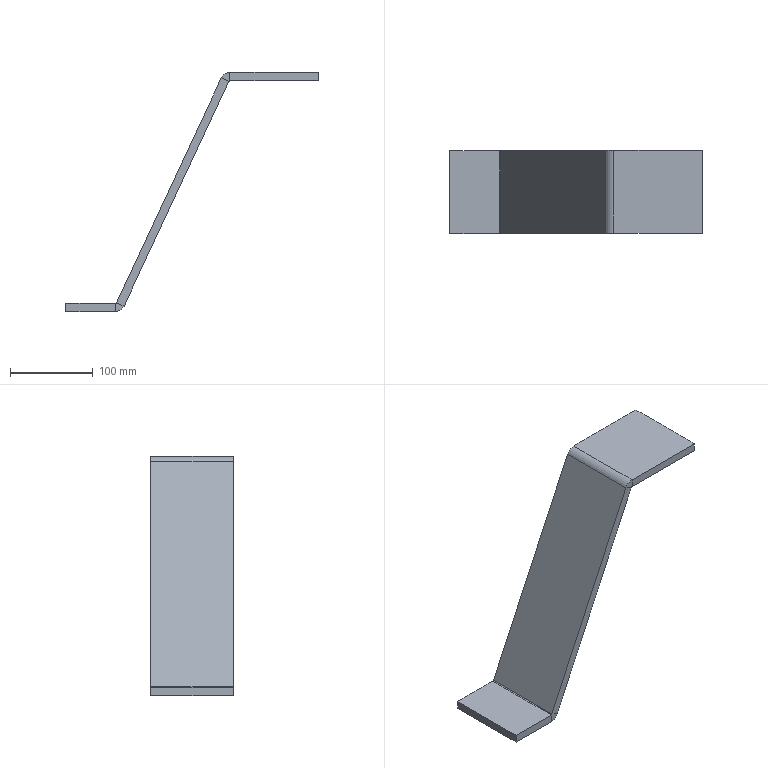Part | STEP file | B1 | 1 solid | 22 faces | box 305.057 x 100 x 289.003 mm | volume 480985 mm3 | plane 18 | cylinder 4 | commonest cylinder face diameters 3 x2 23 x2
STEP:
#1=CARTESIAN_POINT('',(0.,0.,0.));
#2=DIRECTION('',(0.,0.,1.));
#3=DIRECTION('',(1.,0.,0.));
#4=AXIS2_PLACEMENT_3D('',#1,#2,#3);
#5=CARTESIAN_POINT('',(0.,100.,0.));
#6=VERTEX_POINT('',#5);
#7=CARTESIAN_POINT('',(0.,0.,0.));
#8=VERTEX_POINT('',#7);
#9=CARTESIAN_POINT('',(0.,100.,0.));
#10=DIRECTION('',(0.,-1.,0.));
#11=VECTOR('',#10,1.);
#12=LINE('',#9,#11);
#13=CARTESIAN_POINT('',(0.,100.,-10.));
#14=DIRECTION('',(-1.,0.,0.));
#15=DIRECTION('',(0.,-1.,0.));
#16=AXIS2_PLACEMENT_3D('',#13,#14,#15);
#17=PLANE('',#16);
#18=CARTESIAN_POINT('',(0.,10.));
#19=DIRECTION('',(1.,0.));
#20=VECTOR('',#19,1.);
#21=LINE('',#18,#20);
#22=(GEOMETRIC_REPRESENTATION_CONTEXT(2)PARAMETRIC_REPRESENTATION_CONTEXT()REPRESENTATION_CONTEXT('',''));
#23=DEFINITIONAL_REPRESENTATION('',(#21),#22);
#24=PCURVE('',#17,#23);
#25=CARTESIAN_POINT('',(0.,0.,0.));
#26=DIRECTION('',(0.,0.,1.));
#27=DIRECTION('',(1.,0.,0.));
#28=AXIS2_PLACEMENT_3D('',#25,#26,#27);
#29=PLANE('',#28);
#30=CARTESIAN_POINT('',(0.,100.));
#31=DIRECTION('',(0.,-1.));
#32=VECTOR('',#31,1.);
#33=LINE('',#30,#32);
#34=(GEOMETRIC_REPRESENTATION_CONTEXT(2)PARAMETRIC_REPRESENTATION_CONTEXT()REPRESENTATION_CONTEXT('',''));
#35=DEFINITIONAL_REPRESENTATION('',(#33),#34);
#36=PCURVE('',#29,#35);
#37=SURFACE_CURVE('',#12,(#24,#36),.PCURVE_S1.);
#38=EDGE_CURVE('',#6,#8,#37,.T.);
#39=ORIENTED_EDGE('',*,*,#38,.F.);
#40=CARTESIAN_POINT('',(0.,100.,-10.));
#41=VERTEX_POINT('',#40);
#42=CARTESIAN_POINT('',(0.,100.,-10.));
#43=DIRECTION('',(0.,0.,1.));
#44=VECTOR('',#43,1.);
#45=LINE('',#42,#44);
#46=CARTESIAN_POINT('',(0.,0.));
#47=DIRECTION('',(0.,1.));
#48=VECTOR('',#47,1.);
#49=LINE('',#46,#48);
#50=(GEOMETRIC_REPRESENTATION_CONTEXT(2)PARAMETRIC_REPRESENTATION_CONTEXT()REPRESENTATION_CONTEXT('',''));
#51=DEFINITIONAL_REPRESENTATION('',(#49),#50);
#52=PCURVE('',#17,#51);
#53=CARTESIAN_POINT('',(0.,100.,-10.));
#54=DIRECTION('',(0.,1.,0.));
#55=DIRECTION('',(-1.,0.,0.));
#56=AXIS2_PLACEMENT_3D('',#53,#54,#55);
#57=PLANE('',#56);
#58=CARTESIAN_POINT('',(0.,0.));
#59=DIRECTION('',(0.,1.));
#60=VECTOR('',#59,1.);
#61=LINE('',#58,#60);
#62=(GEOMETRIC_REPRESENTATION_CONTEXT(2)PARAMETRIC_REPRESENTATION_CONTEXT()REPRESENTATION_CONTEXT('',''));
#63=DEFINITIONAL_REPRESENTATION('',(#61),#62);
#64=PCURVE('',#57,#63);
#65=SURFACE_CURVE('',#45,(#52,#64),.PCURVE_S1.);
#66=EDGE_CURVE('',#41,#6,#65,.T.);
#67=ORIENTED_EDGE('',*,*,#66,.F.);
#68=CARTESIAN_POINT('',(0.,0.,-10.));
#69=VERTEX_POINT('',#68);
#70=CARTESIAN_POINT('',(0.,100.,-10.));
#71=DIRECTION('',(0.,-1.,0.));
#72=VECTOR('',#71,1.);
#73=LINE('',#70,#72);
#74=CARTESIAN_POINT('',(0.,0.));
#75=DIRECTION('',(1.,0.));
#76=VECTOR('',#75,1.);
#77=LINE('',#74,#76);
#78=(GEOMETRIC_REPRESENTATION_CONTEXT(2)PARAMETRIC_REPRESENTATION_CONTEXT()REPRESENTATION_CONTEXT('',''));
#79=DEFINITIONAL_REPRESENTATION('',(#77),#78);
#80=PCURVE('',#17,#79);
#81=CARTESIAN_POINT('',(0.,0.,-10.));
#82=DIRECTION('',(0.,0.,1.));
#83=DIRECTION('',(1.,0.,0.));
#84=AXIS2_PLACEMENT_3D('',#81,#82,#83);
#85=PLANE('',#84);
#86=CARTESIAN_POINT('',(0.,100.));
#87=DIRECTION('',(0.,-1.));
#88=VECTOR('',#87,1.);
#89=LINE('',#86,#88);
#90=(GEOMETRIC_REPRESENTATION_CONTEXT(2)PARAMETRIC_REPRESENTATION_CONTEXT()REPRESENTATION_CONTEXT('',''));
#91=DEFINITIONAL_REPRESENTATION('',(#89),#90);
#92=PCURVE('',#85,#91);
#93=SURFACE_CURVE('',#73,(#80,#92),.PCURVE_S1.);
#94=EDGE_CURVE('',#41,#69,#93,.T.);
#95=ORIENTED_EDGE('',*,*,#94,.T.);
#96=CARTESIAN_POINT('',(0.,0.,-10.));
#97=DIRECTION('',(0.,0.,1.));
#98=VECTOR('',#97,1.);
#99=LINE('',#96,#98);
#100=CARTESIAN_POINT('',(100.,0.));
#101=DIRECTION('',(0.,1.));
#102=VECTOR('',#101,1.);
#103=LINE('',#100,#102);
#104=(GEOMETRIC_REPRESENTATION_CONTEXT(2)PARAMETRIC_REPRESENTATION_CONTEXT()REPRESENTATION_CONTEXT('',''));
#105=DEFINITIONAL_REPRESENTATION('',(#103),#104);
#106=PCURVE('',#17,#105);
#107=CARTESIAN_POINT('',(0.,0.,-10.));
#108=DIRECTION('',(0.,-1.,0.));
#109=DIRECTION('',(1.,0.,0.));
#110=AXIS2_PLACEMENT_3D('',#107,#108,#109);
#111=PLANE('',#110);
#112=CARTESIAN_POINT('',(0.,0.));
#113=DIRECTION('',(0.,1.));
#114=VECTOR('',#113,1.);
#115=LINE('',#112,#114);
#116=(GEOMETRIC_REPRESENTATION_CONTEXT(2)PARAMETRIC_REPRESENTATION_CONTEXT()REPRESENTATION_CONTEXT('',''));
#117=DEFINITIONAL_REPRESENTATION('',(#115),#116);
#118=PCURVE('',#111,#117);
#119=SURFACE_CURVE('',#99,(#106,#118),.PCURVE_S1.);
#120=EDGE_CURVE('',#69,#8,#119,.T.);
#121=ORIENTED_EDGE('',*,*,#120,.T.);
#122=EDGE_LOOP('',(#39,#67,#95,#121));
#123=FACE_BOUND('',#122,.T.);
#124=ADVANCED_FACE('',(#123),#17,.T.);
#125=CARTESIAN_POINT('',(60.,100.,0.));
#126=VERTEX_POINT('',#125);
#127=CARTESIAN_POINT('',(0.,100.,0.));
#128=DIRECTION('',(-1.,0.,0.));
#129=VECTOR('',#128,1.);
#130=LINE('',#127,#129);
#131=CARTESIAN_POINT('',(0.,10.));
#132=DIRECTION('',(1.,0.));
#133=VECTOR('',#132,1.);
#134=LINE('',#131,#133);
#135=(GEOMETRIC_REPRESENTATION_CONTEXT(2)PARAMETRIC_REPRESENTATION_CONTEXT()REPRESENTATION_CONTEXT('',''));
#136=DEFINITIONAL_REPRESENTATION('',(#134),#135);
#137=PCURVE('',#57,#136);
#138=CARTESIAN_POINT('',(0.,100.));
#139=DIRECTION('',(-1.,0.));
#140=VECTOR('',#139,1.);
#141=LINE('',#138,#140);
#142=(GEOMETRIC_REPRESENTATION_CONTEXT(2)PARAMETRIC_REPRESENTATION_CONTEXT()REPRESENTATION_CONTEXT('',''));
#143=DEFINITIONAL_REPRESENTATION('',(#141),#142);
#144=PCURVE('',#29,#143);
#145=SURFACE_CURVE('',#130,(#137,#144),.PCURVE_S1.);
#146=EDGE_CURVE('',#126,#6,#145,.T.);
#147=ORIENTED_EDGE('',*,*,#146,.F.);
#148=CARTESIAN_POINT('',(60.,100.,-10.));
#149=VERTEX_POINT('',#148);
#150=CARTESIAN_POINT('',(60.,100.,-10.));
#151=DIRECTION('',(0.,0.,1.));
#152=VECTOR('',#151,1.);
#153=LINE('',#150,#152);
#154=CARTESIAN_POINT('',(-60.,0.));
#155=DIRECTION('',(0.,1.));
#156=VECTOR('',#155,1.);
#157=LINE('',#154,#156);
#158=(GEOMETRIC_REPRESENTATION_CONTEXT(2)PARAMETRIC_REPRESENTATION_CONTEXT()REPRESENTATION_CONTEXT('',''));
#159=DEFINITIONAL_REPRESENTATION('',(#157),#158);
#160=PCURVE('',#57,#159);
#161=CARTESIAN_POINT('',(60.,100.,1.5));
#162=DIRECTION('',(0.,-1.,0.));
#163=DIRECTION('',(1.,0.,0.));
#164=AXIS2_PLACEMENT_3D('',#161,#162,#163);
#165=PLANE('',#164);
#166=CARTESIAN_POINT('',(0.,-11.5));
#167=DIRECTION('',(0.,1.));
#168=VECTOR('',#167,1.);
#169=LINE('',#166,#168);
#170=(GEOMETRIC_REPRESENTATION_CONTEXT(2)PARAMETRIC_REPRESENTATION_CONTEXT()REPRESENTATION_CONTEXT('',''));
#171=DEFINITIONAL_REPRESENTATION('',(#169),#170);
#172=PCURVE('',#165,#171);
#173=SURFACE_CURVE('',#153,(#160,#172),.PCURVE_S1.);
#174=EDGE_CURVE('',#149,#126,#173,.T.);
#175=ORIENTED_EDGE('',*,*,#174,.F.);
#176=CARTESIAN_POINT('',(0.,100.,-10.));
#177=DIRECTION('',(-1.,0.,0.));
#178=VECTOR('',#177,1.);
#179=LINE('',#176,#178);
#180=CARTESIAN_POINT('',(0.,0.));
#181=DIRECTION('',(1.,0.));
#182=VECTOR('',#181,1.);
#183=LINE('',#180,#182);
#184=(GEOMETRIC_REPRESENTATION_CONTEXT(2)PARAMETRIC_REPRESENTATION_CONTEXT()REPRESENTATION_CONTEXT('',''));
#185=DEFINITIONAL_REPRESENTATION('',(#183),#184);
#186=PCURVE('',#57,#185);
#187=CARTESIAN_POINT('',(0.,100.));
#188=DIRECTION('',(-1.,0.));
#189=VECTOR('',#188,1.);
#190=LINE('',#187,#189);
#191=(GEOMETRIC_REPRESENTATION_CONTEXT(2)PARAMETRIC_REPRESENTATION_CONTEXT()REPRESENTATION_CONTEXT('',''));
#192=DEFINITIONAL_REPRESENTATION('',(#190),#191);
#193=PCURVE('',#85,#192);
#194=SURFACE_CURVE('',#179,(#186,#193),.PCURVE_S1.);
#195=EDGE_CURVE('',#149,#41,#194,.T.);
#196=ORIENTED_EDGE('',*,*,#195,.T.);
#197=ORIENTED_EDGE('',*,*,#66,.T.);
#198=EDGE_LOOP('',(#147,#175,#196,#197));
#199=FACE_BOUND('',#198,.T.);
#200=ADVANCED_FACE('',(#199),#57,.T.);
#201=CARTESIAN_POINT('',(60.,0.,0.));
#202=VERTEX_POINT('',#201);
#203=CARTESIAN_POINT('',(0.,0.,0.));
#204=DIRECTION('',(1.,0.,0.));
#205=VECTOR('',#204,1.);
#206=LINE('',#203,#205);
#207=CARTESIAN_POINT('',(0.,10.));
#208=DIRECTION('',(1.,0.));
#209=VECTOR('',#208,1.);
#210=LINE('',#207,#209);
#211=(GEOMETRIC_REPRESENTATION_CONTEXT(2)PARAMETRIC_REPRESENTATION_CONTEXT()REPRESENTATION_CONTEXT('',''));
#212=DEFINITIONAL_REPRESENTATION('',(#210),#211);
#213=PCURVE('',#111,#212);
#214=CARTESIAN_POINT('',(0.,0.));
#215=DIRECTION('',(1.,0.));
#216=VECTOR('',#215,1.);
#217=LINE('',#214,#216);
#218=(GEOMETRIC_REPRESENTATION_CONTEXT(2)PARAMETRIC_REPRESENTATION_CONTEXT()REPRESENTATION_CONTEXT('',''));
#219=DEFINITIONAL_REPRESENTATION('',(#217),#218);
#220=PCURVE('',#29,#219);
#221=SURFACE_CURVE('',#206,(#213,#220),.PCURVE_S1.);
#222=EDGE_CURVE('',#8,#202,#221,.T.);
#223=ORIENTED_EDGE('',*,*,#222,.F.);
#224=ORIENTED_EDGE('',*,*,#120,.F.);
#225=CARTESIAN_POINT('',(60.,0.,-10.));
#226=VERTEX_POINT('',#225);
#227=CARTESIAN_POINT('',(0.,0.,-10.));
#228=DIRECTION('',(1.,0.,0.));
#229=VECTOR('',#228,1.);
#230=LINE('',#227,#229);
#231=CARTESIAN_POINT('',(0.,0.));
#232=DIRECTION('',(1.,0.));
#233=VECTOR('',#232,1.);
#234=LINE('',#231,#233);
#235=(GEOMETRIC_REPRESENTATION_CONTEXT(2)PARAMETRIC_REPRESENTATION_CONTEXT()REPRESENTATION_CONTEXT('',''));
#236=DEFINITIONAL_REPRESENTATION('',(#234),#235);
#237=PCURVE('',#111,#236);
#238=CARTESIAN_POINT('',(0.,0.));
#239=DIRECTION('',(1.,0.));
#240=VECTOR('',#239,1.);
#241=LINE('',#238,#240);
#242=(GEOMETRIC_REPRESENTATION_CONTEXT(2)PARAMETRIC_REPRESENTATION_CONTEXT()REPRESENTATION_CONTEXT('',''));
#243=DEFINITIONAL_REPRESENTATION('',(#241),#242);
#244=PCURVE('',#85,#243);
#245=SURFACE_CURVE('',#230,(#237,#244),.PCURVE_S1.);
#246=EDGE_CURVE('',#69,#226,#245,.T.);
#247=ORIENTED_EDGE('',*,*,#246,.T.);
#248=CARTESIAN_POINT('',(60.,0.,-10.));
#249=DIRECTION('',(0.,0.,1.));
#250=VECTOR('',#249,1.);
#251=LINE('',#248,#250);
#252=CARTESIAN_POINT('',(60.,0.));
#253=DIRECTION('',(0.,1.));
#254=VECTOR('',#253,1.);
#255=LINE('',#252,#254);
#256=(GEOMETRIC_REPRESENTATION_CONTEXT(2)PARAMETRIC_REPRESENTATION_CONTEXT()REPRESENTATION_CONTEXT('',''));
#257=DEFINITIONAL_REPRESENTATION('',(#255),#256);
#258=PCURVE('',#111,#257);
#259=CARTESIAN_POINT('',(60.,0.,1.5));
#260=DIRECTION('',(0.,-1.,0.));
#261=DIRECTION('',(1.,0.,0.));
#262=AXIS2_PLACEMENT_3D('',#259,#260,#261);
#263=PLANE('',#262);
#264=CARTESIAN_POINT('',(0.,-11.5));
#265=DIRECTION('',(0.,1.));
#266=VECTOR('',#265,1.);
#267=LINE('',#264,#266);
#268=(GEOMETRIC_REPRESENTATION_CONTEXT(2)PARAMETRIC_REPRESENTATION_CONTEXT()REPRESENTATION_CONTEXT('',''));
#269=DEFINITIONAL_REPRESENTATION('',(#267),#268);
#270=PCURVE('',#263,#269);
#271=SURFACE_CURVE('',#251,(#258,#270),.PCURVE_S1.);
#272=EDGE_CURVE('',#226,#202,#271,.T.);
#273=ORIENTED_EDGE('',*,*,#272,.T.);
#274=EDGE_LOOP('',(#223,#224,#247,#273));
#275=FACE_BOUND('',#274,.T.);
#276=ADVANCED_FACE('',(#275),#111,.T.);
#277=ORIENTED_EDGE('',*,*,#94,.F.);
#278=ORIENTED_EDGE('',*,*,#195,.F.);
#279=CARTESIAN_POINT('',(60.,100.,-10.));
#280=DIRECTION('',(0.,1.,0.));
#281=VECTOR('',#280,1.);
#282=LINE('',#279,#281);
#283=CARTESIAN_POINT('',(60.,100.));
#284=DIRECTION('',(0.,1.));
#285=VECTOR('',#284,1.);
#286=LINE('',#283,#285);
#287=(GEOMETRIC_REPRESENTATION_CONTEXT(2)PARAMETRIC_REPRESENTATION_CONTEXT()REPRESENTATION_CONTEXT('',''));
#288=DEFINITIONAL_REPRESENTATION('',(#286),#287);
#289=PCURVE('',#85,#288);
#290=CARTESIAN_POINT('',(60.,100.,1.5));
#291=DIRECTION('',(0.,1.,0.));
#292=DIRECTION('',(0.9063,0.,-0.4226));
#293=AXIS2_PLACEMENT_3D('',#290,#291,#292);
#294=CYLINDRICAL_SURFACE('',#293,11.5);
#295=CARTESIAN_POINT('',(1.134,0.));
#296=DIRECTION('',(0.,1.));
#297=VECTOR('',#296,1.);
#298=LINE('',#295,#297);
#299=(GEOMETRIC_REPRESENTATION_CONTEXT(2)PARAMETRIC_REPRESENTATION_CONTEXT()REPRESENTATION_CONTEXT('',''));
#300=DEFINITIONAL_REPRESENTATION('',(#298),#299);
#301=PCURVE('',#294,#300);
#302=SURFACE_CURVE('',#282,(#289,#301),.PCURVE_S1.);
#303=EDGE_CURVE('',#226,#149,#302,.T.);
#304=ORIENTED_EDGE('',*,*,#303,.F.);
#305=ORIENTED_EDGE('',*,*,#246,.F.);
#306=EDGE_LOOP('',(#277,#278,#304,#305));
#307=FACE_BOUND('',#306,.T.);
#308=ADVANCED_FACE('',(#307),#85,.F.);
#309=ORIENTED_EDGE('',*,*,#38,.T.);
#310=ORIENTED_EDGE('',*,*,#222,.T.);
#311=CARTESIAN_POINT('',(60.,100.,0.));
#312=DIRECTION('',(0.,1.,0.));
#313=VECTOR('',#312,1.);
#314=LINE('',#311,#313);
#315=CARTESIAN_POINT('',(60.,100.));
#316=DIRECTION('',(0.,1.));
#317=VECTOR('',#316,1.);
#318=LINE('',#315,#317);
#319=(GEOMETRIC_REPRESENTATION_CONTEXT(2)PARAMETRIC_REPRESENTATION_CONTEXT()REPRESENTATION_CONTEXT('',''));
#320=DEFINITIONAL_REPRESENTATION('',(#318),#319);
#321=PCURVE('',#29,#320);
#322=CARTESIAN_POINT('',(60.,100.,1.5));
#323=DIRECTION('',(0.,1.,0.));
#324=DIRECTION('',(0.9063,0.,-0.4226));
#325=AXIS2_PLACEMENT_3D('',#322,#323,#324);
#326=CYLINDRICAL_SURFACE('',#325,1.5);
#327=CARTESIAN_POINT('',(1.134,0.));
#328=DIRECTION('',(0.,1.));
#329=VECTOR('',#328,1.);
#330=LINE('',#327,#329);
#331=(GEOMETRIC_REPRESENTATION_CONTEXT(2)PARAMETRIC_REPRESENTATION_CONTEXT()REPRESENTATION_CONTEXT('',''));
#332=DEFINITIONAL_REPRESENTATION('',(#330),#331);
#333=PCURVE('',#326,#332);
#334=SURFACE_CURVE('',#314,(#321,#333),.PCURVE_S1.);
#335=EDGE_CURVE('',#202,#126,#334,.T.);
#336=ORIENTED_EDGE('',*,*,#335,.T.);
#337=ORIENTED_EDGE('',*,*,#146,.T.);
#338=EDGE_LOOP('',(#309,#310,#336,#337));
#339=FACE_BOUND('',#338,.T.);
#340=ADVANCED_FACE('',(#339),#29,.T.);
#341=CARTESIAN_POINT('',(61.359,0.,0.8661));
#342=VERTEX_POINT('',#341);
#343=CARTESIAN_POINT('',(70.423,0.,-3.36));
#344=VERTEX_POINT('',#343);
#345=CARTESIAN_POINT('',(70.423,0.,-3.36));
#346=DIRECTION('',(0.9063,0.,-0.4226));
#347=VECTOR('',#346,1.);
#348=LINE('',#345,#347);
#349=CARTESIAN_POINT('',(10.423,-4.86));
#350=DIRECTION('',(0.9063,-0.4226));
#351=VECTOR('',#350,1.);
#352=LINE('',#349,#351);
#353=(GEOMETRIC_REPRESENTATION_CONTEXT(2)PARAMETRIC_REPRESENTATION_CONTEXT()REPRESENTATION_CONTEXT('',''));
#354=DEFINITIONAL_REPRESENTATION('',(#352),#353);
#355=PCURVE('',#263,#354);
#356=CARTESIAN_POINT('',(70.019,0.,-4.226));
#357=DIRECTION('',(0.,1.,0.));
#358=DIRECTION('',(-1.,0.,0.));
#359=AXIS2_PLACEMENT_3D('',#356,#357,#358);
#360=PLANE('',#359);
#361=CARTESIAN_POINT('',(-0.4039,0.8661));
#362=DIRECTION('',(-0.9063,-0.4226));
#363=VECTOR('',#362,1.);
#364=LINE('',#361,#363);
#365=(GEOMETRIC_REPRESENTATION_CONTEXT(2)PARAMETRIC_REPRESENTATION_CONTEXT()REPRESENTATION_CONTEXT('',''));
#366=DEFINITIONAL_REPRESENTATION('',(#364),#365);
#367=PCURVE('',#360,#366);
#368=SURFACE_CURVE('',#348,(#355,#367),.PCURVE_S1.);
#369=EDGE_CURVE('',#342,#344,#368,.T.);
#370=ORIENTED_EDGE('',*,*,#369,.F.);
#371=CARTESIAN_POINT('',(60.,0.,1.5));
#372=DIRECTION('',(0.,-1.,0.));
#373=DIRECTION('',(-1.,0.,0.));
#374=AXIS2_PLACEMENT_3D('',#371,#372,#373);
#375=CIRCLE('',#374,1.5);
#376=CARTESIAN_POINT('',(0.,0.));
#377=DIRECTION('',(-1.,0.));
#378=AXIS2_PLACEMENT_2D('',#376,#377);
#379=CIRCLE('',#378,1.5);
#380=(GEOMETRIC_REPRESENTATION_CONTEXT(2)PARAMETRIC_REPRESENTATION_CONTEXT()REPRESENTATION_CONTEXT('',''));
#381=DEFINITIONAL_REPRESENTATION('',(#379),#380);
#382=PCURVE('',#263,#381);
#383=CARTESIAN_POINT('',(2.705,-100.));
#384=DIRECTION('',(-1.,0.));
#385=VECTOR('',#384,1.);
#386=LINE('',#383,#385);
#387=(GEOMETRIC_REPRESENTATION_CONTEXT(2)PARAMETRIC_REPRESENTATION_CONTEXT()REPRESENTATION_CONTEXT('',''));
#388=DEFINITIONAL_REPRESENTATION('',(#386),#387);
#389=PCURVE('',#326,#388);
#390=SURFACE_CURVE('',#375,(#382,#389),.PCURVE_S1.);
#391=EDGE_CURVE('',#202,#342,#390,.T.);
#392=ORIENTED_EDGE('',*,*,#391,.F.);
#393=ORIENTED_EDGE('',*,*,#272,.F.);
#394=CARTESIAN_POINT('',(60.,0.,1.5));
#395=DIRECTION('',(0.,-1.,0.));
#396=DIRECTION('',(-1.,0.,0.));
#397=AXIS2_PLACEMENT_3D('',#394,#395,#396);
#398=CIRCLE('',#397,11.5);
#399=CARTESIAN_POINT('',(0.,0.));
#400=DIRECTION('',(-1.,0.));
#401=AXIS2_PLACEMENT_2D('',#399,#400);
#402=CIRCLE('',#401,11.5);
#403=(GEOMETRIC_REPRESENTATION_CONTEXT(2)PARAMETRIC_REPRESENTATION_CONTEXT()REPRESENTATION_CONTEXT('',''));
#404=DEFINITIONAL_REPRESENTATION('',(#402),#403);
#405=PCURVE('',#263,#404);
#406=CARTESIAN_POINT('',(2.705,-100.));
#407=DIRECTION('',(-1.,0.));
#408=VECTOR('',#407,1.);
#409=LINE('',#406,#408);
#410=(GEOMETRIC_REPRESENTATION_CONTEXT(2)PARAMETRIC_REPRESENTATION_CONTEXT()REPRESENTATION_CONTEXT('',''));
#411=DEFINITIONAL_REPRESENTATION('',(#409),#410);
#412=PCURVE('',#294,#411);
#413=SURFACE_CURVE('',#398,(#405,#412),.PCURVE_S1.);
#414=EDGE_CURVE('',#226,#344,#413,.T.);
#415=ORIENTED_EDGE('',*,*,#414,.T.);
#416=EDGE_LOOP('',(#370,#392,#393,#415));
#417=FACE_BOUND('',#416,.T.);
#418=ADVANCED_FACE('',(#417),#263,.T.);
#419=CARTESIAN_POINT('',(61.359,100.,0.8661));
#420=VERTEX_POINT('',#419);
#421=CARTESIAN_POINT('',(60.,100.,1.5));
#422=DIRECTION('',(0.,1.,0.));
#423=DIRECTION('',(-1.,0.,0.));
#424=AXIS2_PLACEMENT_3D('',#421,#422,#423);
#425=CIRCLE('',#424,1.5);
#426=CARTESIAN_POINT('',(-1.5,0.));
#427=CARTESIAN_POINT('',(-1.5,2.598));
#428=CARTESIAN_POINT('',(0.75,1.299));
#429=CARTESIAN_POINT('',(3.,0.));
#430=CARTESIAN_POINT('',(0.75,-1.299));
#431=CARTESIAN_POINT('',(-1.5,-2.598));
#432=CARTESIAN_POINT('',(-1.5,0.));
#433=(BOUNDED_CURVE()B_SPLINE_CURVE(2,(#426,#427,#428,#429,#430,#431,#432),.UNSPECIFIED.,.T.,.F.)B_SPLINE_CURVE_WITH_KNOTS((1,2,2,2,2,1),(-2.094,0.,2.094,4.189,6.283,8.378),.UNSPECIFIED.)CURVE()GEOMETRIC_REPRESENTATION_ITEM()RATIONAL_B_SPLINE_CURVE((1.,0.5,1.,0.5,1.,0.5,1.))REPRESENTATION_ITEM(''));
#434=(GEOMETRIC_REPRESENTATION_CONTEXT(2)PARAMETRIC_REPRESENTATION_CONTEXT()REPRESENTATION_CONTEXT('',''));
#435=DEFINITIONAL_REPRESENTATION('',(#433),#434);
#436=PCURVE('',#165,#435);
#437=CARTESIAN_POINT('',(-3.578,0.));
#438=DIRECTION('',(1.,0.));
#439=VECTOR('',#438,1.);
#440=LINE('',#437,#439);
#441=(GEOMETRIC_REPRESENTATION_CONTEXT(2)PARAMETRIC_REPRESENTATION_CONTEXT()REPRESENTATION_CONTEXT('',''));
#442=DEFINITIONAL_REPRESENTATION('',(#440),#441);
#443=PCURVE('',#326,#442);
#444=SURFACE_CURVE('',#425,(#436,#443),.PCURVE_S1.);
#445=EDGE_CURVE('',#420,#126,#444,.T.);
#446=ORIENTED_EDGE('',*,*,#445,.F.);
#447=CARTESIAN_POINT('',(70.423,100.,-3.36));
#448=VERTEX_POINT('',#447);
#449=CARTESIAN_POINT('',(61.359,100.,0.8661));
#450=DIRECTION('',(0.9063,0.,-0.4226));
#451=VECTOR('',#450,1.);
#452=LINE('',#449,#451);
#453=CARTESIAN_POINT('',(1.359,-0.6339));
#454=DIRECTION('',(0.9063,-0.4226));
#455=VECTOR('',#454,1.);
#456=LINE('',#453,#455);
#457=(GEOMETRIC_REPRESENTATION_CONTEXT(2)PARAMETRIC_REPRESENTATION_CONTEXT()REPRESENTATION_CONTEXT('',''));
#458=DEFINITIONAL_REPRESENTATION('',(#456),#457);
#459=PCURVE('',#165,#458);
#460=CARTESIAN_POINT('',(197.024,100.,268.137));
#461=DIRECTION('',(0.,-1.,0.));
#462=DIRECTION('',(1.,0.,0.));
#463=AXIS2_PLACEMENT_3D('',#460,#461,#462);
#464=PLANE('',#463);
#465=CARTESIAN_POINT('',(-135.664,-267.271));
#466=DIRECTION('',(0.9063,-0.4226));
#467=VECTOR('',#466,1.);
#468=LINE('',#465,#467);
#469=(GEOMETRIC_REPRESENTATION_CONTEXT(2)PARAMETRIC_REPRESENTATION_CONTEXT()REPRESENTATION_CONTEXT('',''));
#470=DEFINITIONAL_REPRESENTATION('',(#468),#469);
#471=PCURVE('',#464,#470);
#472=SURFACE_CURVE('',#452,(#459,#471),.PCURVE_S1.);
#473=EDGE_CURVE('',#420,#448,#472,.T.);
#474=ORIENTED_EDGE('',*,*,#473,.T.);
#475=CARTESIAN_POINT('',(60.,100.,1.5));
#476=DIRECTION('',(0.,1.,0.));
#477=DIRECTION('',(-1.,0.,0.));
#478=AXIS2_PLACEMENT_3D('',#475,#476,#477);
#479=CIRCLE('',#478,11.5);
#480=CARTESIAN_POINT('',(-11.5,0.));
#481=CARTESIAN_POINT('',(-11.5,19.919));
#482=CARTESIAN_POINT('',(5.75,9.959));
#483=CARTESIAN_POINT('',(23.,0.));
#484=CARTESIAN_POINT('',(5.75,-9.959));
#485=CARTESIAN_POINT('',(-11.5,-19.919));
#486=CARTESIAN_POINT('',(-11.5,0.));
#487=(BOUNDED_CURVE()B_SPLINE_CURVE(2,(#480,#481,#482,#483,#484,#485,#486),.UNSPECIFIED.,.T.,.F.)B_SPLINE_CURVE_WITH_KNOTS((1,2,2,2,2,1),(-2.094,0.,2.094,4.189,6.283,8.378),.UNSPECIFIED.)CURVE()GEOMETRIC_REPRESENTATION_ITEM()RATIONAL_B_SPLINE_CURVE((1.,0.5,1.,0.5,1.,0.5,1.))REPRESENTATION_ITEM(''));
#488=(GEOMETRIC_REPRESENTATION_CONTEXT(2)PARAMETRIC_REPRESENTATION_CONTEXT()REPRESENTATION_CONTEXT('',''));
#489=DEFINITIONAL_REPRESENTATION('',(#487),#488);
#490=PCURVE('',#165,#489);
#491=CARTESIAN_POINT('',(-3.578,0.));
#492=DIRECTION('',(1.,0.));
#493=VECTOR('',#492,1.);
#494=LINE('',#491,#493);
#495=(GEOMETRIC_REPRESENTATION_CONTEXT(2)PARAMETRIC_REPRESENTATION_CONTEXT()REPRESENTATION_CONTEXT('',''));
#496=DEFINITIONAL_REPRESENTATION('',(#494),#495);
#497=PCURVE('',#294,#496);
#498=SURFACE_CURVE('',#479,(#490,#497),.PCURVE_S1.);
#499=EDGE_CURVE('',#448,#149,#498,.T.);
#500=ORIENTED_EDGE('',*,*,#499,.T.);
#501=ORIENTED_EDGE('',*,*,#174,.T.);
#502=EDGE_LOOP('',(#446,#474,#500,#501));
#503=FACE_BOUND('',#502,.T.);
#504=ADVANCED_FACE('',(#503),#165,.F.);
#505=ORIENTED_EDGE('',*,*,#303,.T.);
#506=ORIENTED_EDGE('',*,*,#499,.F.);
#507=CARTESIAN_POINT('',(70.423,0.,-3.36));
#508=DIRECTION('',(0.,-1.,0.));
#509=VECTOR('',#508,1.);
#510=LINE('',#507,#509);
#511=CARTESIAN_POINT('',(0.,-100.));
#512=DIRECTION('',(0.,-1.));
#513=VECTOR('',#512,1.);
#514=LINE('',#511,#513);
#515=(GEOMETRIC_REPRESENTATION_CONTEXT(2)PARAMETRIC_REPRESENTATION_CONTEXT()REPRESENTATION_CONTEXT('',''));
#516=DEFINITIONAL_REPRESENTATION('',(#514),#515);
#517=PCURVE('',#294,#516);
#518=CARTESIAN_POINT('',(59.302,0.,-27.208));
#519=DIRECTION('',(-0.9063,0.,0.4226));
#520=DIRECTION('',(0.4226,0.,0.9063));
#521=AXIS2_PLACEMENT_3D('',#518,#519,#520);
#522=PLANE('',#521);
#523=CARTESIAN_POINT('',(26.313,0.));
#524=DIRECTION('',(0.,-1.));
#525=VECTOR('',#524,1.);
#526=LINE('',#523,#525);
#527=(GEOMETRIC_REPRESENTATION_CONTEXT(2)PARAMETRIC_REPRESENTATION_CONTEXT()REPRESENTATION_CONTEXT('',''));
#528=DEFINITIONAL_REPRESENTATION('',(#526),#527);
#529=PCURVE('',#522,#528);
#530=SURFACE_CURVE('',#510,(#517,#529),.PCURVE_S1.);
#531=EDGE_CURVE('',#448,#344,#530,.T.);
#532=ORIENTED_EDGE('',*,*,#531,.T.);
#533=ORIENTED_EDGE('',*,*,#414,.F.);
#534=EDGE_LOOP('',(#505,#506,#532,#533));
#535=FACE_BOUND('',#534,.T.);
#536=ADVANCED_FACE('',(#535),#294,.T.);
#537=ORIENTED_EDGE('',*,*,#445,.F.);
#538=CARTESIAN_POINT('',(61.359,0.,0.8661));
#539=DIRECTION('',(0.,1.,0.));
#540=VECTOR('',#539,1.);
#541=LINE('',#538,#540);
#542=CARTESIAN_POINT('',(0.,-100.));
#543=DIRECTION('',(0.,1.));
#544=VECTOR('',#543,1.);
#545=LINE('',#542,#544);
#546=(GEOMETRIC_REPRESENTATION_CONTEXT(2)PARAMETRIC_REPRESENTATION_CONTEXT()REPRESENTATION_CONTEXT('',''));
#547=DEFINITIONAL_REPRESENTATION('',(#545),#546);
#548=PCURVE('',#326,#547);
#549=CARTESIAN_POINT('',(50.239,0.,-22.981));
#550=DIRECTION('',(-0.9063,0.,0.4226));
#551=DIRECTION('',(0.4226,0.,0.9063));
#552=AXIS2_PLACEMENT_3D('',#549,#550,#551);
#553=PLANE('',#552);
#554=CARTESIAN_POINT('',(26.313,0.));
#555=DIRECTION('',(0.,1.));
#556=VECTOR('',#555,1.);
#557=LINE('',#554,#556);
#558=(GEOMETRIC_REPRESENTATION_CONTEXT(2)PARAMETRIC_REPRESENTATION_CONTEXT()REPRESENTATION_CONTEXT('',''));
#559=DEFINITIONAL_REPRESENTATION('',(#557),#558);
#560=PCURVE('',#553,#559);
#561=SURFACE_CURVE('',#541,(#548,#560),.PCURVE_S1.);
#562=EDGE_CURVE('',#342,#420,#561,.T.);
#563=ORIENTED_EDGE('',*,*,#562,.F.);
#564=ORIENTED_EDGE('',*,*,#391,.F.);
#565=ORIENTED_EDGE('',*,*,#335,.T.);
#566=EDGE_LOOP('',(#537,#563,#564,#565));
#567=FACE_BOUND('',#566,.F.);
#568=ADVANCED_FACE('',(#567),#326,.F.);
#569=ORIENTED_EDGE('',*,*,#369,.T.);
#570=CARTESIAN_POINT('',(197.024,0.,268.137));
#571=VERTEX_POINT('',#570);
#572=CARTESIAN_POINT('',(59.302,0.,-27.208));
#573=DIRECTION('',(-0.4226,0.,-0.9063));
#574=VECTOR('',#573,1.);
#575=LINE('',#572,#574);
#576=CARTESIAN_POINT('',(10.716,-22.981));
#577=DIRECTION('',(0.4226,-0.9063));
#578=VECTOR('',#577,1.);
#579=LINE('',#576,#578);
#580=(GEOMETRIC_REPRESENTATION_CONTEXT(2)PARAMETRIC_REPRESENTATION_CONTEXT()REPRESENTATION_CONTEXT('',''));
#581=DEFINITIONAL_REPRESENTATION('',(#579),#580);
#582=PCURVE('',#360,#581);
#583=CARTESIAN_POINT('',(0.,0.));
#584=DIRECTION('',(-1.,0.));
#585=VECTOR('',#584,1.);
#586=LINE('',#583,#585);
#587=(GEOMETRIC_REPRESENTATION_CONTEXT(2)PARAMETRIC_REPRESENTATION_CONTEXT()REPRESENTATION_CONTEXT('',''));
#588=DEFINITIONAL_REPRESENTATION('',(#586),#587);
#589=PCURVE('',#522,#588);
#590=SURFACE_CURVE('',#575,(#582,#589),.PCURVE_S1.);
#591=EDGE_CURVE('',#571,#344,#590,.T.);
#592=ORIENTED_EDGE('',*,*,#591,.F.);
#593=CARTESIAN_POINT('',(187.961,0.,272.363));
#594=VERTEX_POINT('',#593);
#595=CARTESIAN_POINT('',(197.024,0.,268.137));
#596=DIRECTION('',(-0.9063,0.,0.4226));
#597=VECTOR('',#596,1.);
#598=LINE('',#595,#597);
#599=CARTESIAN_POINT('',(-127.005,272.363));
#600=DIRECTION('',(0.9063,0.4226));
#601=VECTOR('',#600,1.);
#602=LINE('',#599,#601);
#603=(GEOMETRIC_REPRESENTATION_CONTEXT(2)PARAMETRIC_REPRESENTATION_CONTEXT()REPRESENTATION_CONTEXT('',''));
#604=DEFINITIONAL_REPRESENTATION('',(#602),#603);
#605=PCURVE('',#360,#604);
#606=CARTESIAN_POINT('',(198.383,0.,267.503));
#607=DIRECTION('',(0.,1.,0.));
#608=DIRECTION('',(0.,0.,1.));
#609=AXIS2_PLACEMENT_3D('',#606,#607,#608);
#610=PLANE('',#609);
#611=CARTESIAN_POINT('',(0.6339,-1.359));
#612=DIRECTION('',(0.4226,-0.9063));
#613=VECTOR('',#612,1.);
#614=LINE('',#611,#613);
#615=(GEOMETRIC_REPRESENTATION_CONTEXT(2)PARAMETRIC_REPRESENTATION_CONTEXT()REPRESENTATION_CONTEXT('',''));
#616=DEFINITIONAL_REPRESENTATION('',(#614),#615);
#617=PCURVE('',#610,#616);
#618=SURFACE_CURVE('',#598,(#605,#617),.PCURVE_S1.);
#619=EDGE_CURVE('',#571,#594,#618,.T.);
#620=ORIENTED_EDGE('',*,*,#619,.T.);
#621=CARTESIAN_POINT('',(60.956,0.,0.));
#622=DIRECTION('',(-0.4226,0.,-0.9063));
#623=VECTOR('',#622,1.);
#624=LINE('',#621,#623);
#625=CARTESIAN_POINT('',(9.063,4.226));
#626=DIRECTION('',(0.4226,-0.9063));
#627=VECTOR('',#626,1.);
#628=LINE('',#625,#627);
#629=(GEOMETRIC_REPRESENTATION_CONTEXT(2)PARAMETRIC_REPRESENTATION_CONTEXT()REPRESENTATION_CONTEXT('',''));
#630=DEFINITIONAL_REPRESENTATION('',(#628),#629);
#631=PCURVE('',#360,#630);
#632=CARTESIAN_POINT('',(25.357,0.));
#633=DIRECTION('',(-1.,0.));
#634=VECTOR('',#633,1.);
#635=LINE('',#632,#634);
#636=(GEOMETRIC_REPRESENTATION_CONTEXT(2)PARAMETRIC_REPRESENTATION_CONTEXT()REPRESENTATION_CONTEXT('',''));
#637=DEFINITIONAL_REPRESENTATION('',(#635),#636);
#638=PCURVE('',#553,#637);
#639=SURFACE_CURVE('',#624,(#631,#638),.PCURVE_S1.);
#640=EDGE_CURVE('',#594,#342,#639,.T.);
#641=ORIENTED_EDGE('',*,*,#640,.T.);
#642=EDGE_LOOP('',(#569,#592,#620,#641));
#643=FACE_BOUND('',#642,.T.);
#644=ADVANCED_FACE('',(#643),#360,.F.);
#645=ORIENTED_EDGE('',*,*,#473,.F.);
#646=CARTESIAN_POINT('',(187.961,100.,272.363));
#647=VERTEX_POINT('',#646);
#648=CARTESIAN_POINT('',(187.961,100.,272.363));
#649=DIRECTION('',(0.4226,0.,0.9063));
#650=VECTOR('',#649,1.);
#651=LINE('',#648,#650);
#652=CARTESIAN_POINT('',(-9.063,4.226));
#653=DIRECTION('',(0.4226,0.9063));
#654=VECTOR('',#653,1.);
#655=LINE('',#652,#654);
#656=(GEOMETRIC_REPRESENTATION_CONTEXT(2)PARAMETRIC_REPRESENTATION_CONTEXT()REPRESENTATION_CONTEXT('',''));
#657=DEFINITIONAL_REPRESENTATION('',(#655),#656);
#658=PCURVE('',#464,#657);
#659=CARTESIAN_POINT('',(325.876,100.));
#660=DIRECTION('',(1.,0.));
#661=VECTOR('',#660,1.);
#662=LINE('',#659,#661);
#663=(GEOMETRIC_REPRESENTATION_CONTEXT(2)PARAMETRIC_REPRESENTATION_CONTEXT()REPRESENTATION_CONTEXT('',''));
#664=DEFINITIONAL_REPRESENTATION('',(#662),#663);
#665=PCURVE('',#553,#664);
#666=SURFACE_CURVE('',#651,(#658,#665),.PCURVE_S1.);
#667=EDGE_CURVE('',#420,#647,#666,.T.);
#668=ORIENTED_EDGE('',*,*,#667,.T.);
#669=CARTESIAN_POINT('',(197.024,100.,268.137));
#670=VERTEX_POINT('',#669);
#671=CARTESIAN_POINT('',(197.024,100.,268.137));
#672=DIRECTION('',(-0.9063,0.,0.4226));
#673=VECTOR('',#672,1.);
#674=LINE('',#671,#673);
#675=CARTESIAN_POINT('',(0.,0.));
#676=DIRECTION('',(-0.9063,0.4226));
#677=VECTOR('',#676,1.);
#678=LINE('',#675,#677);
#679=(GEOMETRIC_REPRESENTATION_CONTEXT(2)PARAMETRIC_REPRESENTATION_CONTEXT()REPRESENTATION_CONTEXT('',''));
#680=DEFINITIONAL_REPRESENTATION('',(#678),#679);
#681=PCURVE('',#464,#680);
#682=CARTESIAN_POINT('',(198.383,100.,267.503));
#683=DIRECTION('',(0.,1.,0.));
#684=DIRECTION('',(0.,0.,1.));
#685=AXIS2_PLACEMENT_3D('',#682,#683,#684);
#686=PLANE('',#685);
#687=CARTESIAN_POINT('',(0.6339,-1.359));
#688=DIRECTION('',(0.4226,-0.9063));
#689=VECTOR('',#688,1.);
#690=LINE('',#687,#689);
#691=(GEOMETRIC_REPRESENTATION_CONTEXT(2)PARAMETRIC_REPRESENTATION_CONTEXT()REPRESENTATION_CONTEXT('',''));
#692=DEFINITIONAL_REPRESENTATION('',(#690),#691);
#693=PCURVE('',#686,#692);
#694=SURFACE_CURVE('',#674,(#681,#693),.PCURVE_S1.);
#695=EDGE_CURVE('',#670,#647,#694,.T.);
#696=ORIENTED_EDGE('',*,*,#695,.F.);
#697=CARTESIAN_POINT('',(59.302,100.,-27.208));
#698=DIRECTION('',(0.4226,0.,0.9063));
#699=VECTOR('',#698,1.);
#700=LINE('',#697,#699);
#701=CARTESIAN_POINT('',(-137.721,-295.344));
#702=DIRECTION('',(0.4226,0.9063));
#703=VECTOR('',#702,1.);
#704=LINE('',#701,#703);
#705=(GEOMETRIC_REPRESENTATION_CONTEXT(2)PARAMETRIC_REPRESENTATION_CONTEXT()REPRESENTATION_CONTEXT('',''));
#706=DEFINITIONAL_REPRESENTATION('',(#704),#705);
#707=PCURVE('',#464,#706);
#708=CARTESIAN_POINT('',(0.,100.));
#709=DIRECTION('',(1.,0.));
#710=VECTOR('',#709,1.);
#711=LINE('',#708,#710);
#712=(GEOMETRIC_REPRESENTATION_CONTEXT(2)PARAMETRIC_REPRESENTATION_CONTEXT()REPRESENTATION_CONTEXT('',''));
#713=DEFINITIONAL_REPRESENTATION('',(#711),#712);
#714=PCURVE('',#522,#713);
#715=SURFACE_CURVE('',#700,(#707,#714),.PCURVE_S1.);
#716=EDGE_CURVE('',#448,#670,#715,.T.);
#717=ORIENTED_EDGE('',*,*,#716,.F.);
#718=EDGE_LOOP('',(#645,#668,#696,#717));
#719=FACE_BOUND('',#718,.T.);
#720=ADVANCED_FACE('',(#719),#464,.F.);
#721=ORIENTED_EDGE('',*,*,#531,.F.);
#722=ORIENTED_EDGE('',*,*,#716,.T.);
#723=CARTESIAN_POINT('',(197.024,0.,268.137));
#724=DIRECTION('',(0.,-1.,0.));
#725=VECTOR('',#724,1.);
#726=LINE('',#723,#725);
#727=CARTESIAN_POINT('',(325.876,0.));
#728=DIRECTION('',(0.,-1.));
#729=VECTOR('',#728,1.);
#730=LINE('',#727,#729);
#731=(GEOMETRIC_REPRESENTATION_CONTEXT(2)PARAMETRIC_REPRESENTATION_CONTEXT()REPRESENTATION_CONTEXT('',''));
#732=DEFINITIONAL_REPRESENTATION('',(#730),#731);
#733=PCURVE('',#522,#732);
#734=CARTESIAN_POINT('',(198.383,0.,267.503));
#735=DIRECTION('',(0.,-1.,0.));
#736=DIRECTION('',(0.,0.,1.));
#737=AXIS2_PLACEMENT_3D('',#734,#735,#736);
#738=CYLINDRICAL_SURFACE('',#737,1.5);
#739=CARTESIAN_POINT('',(1.134,0.));
#740=DIRECTION('',(0.,1.));
#741=VECTOR('',#740,1.);
#742=LINE('',#739,#741);
#743=(GEOMETRIC_REPRESENTATION_CONTEXT(2)PARAMETRIC_REPRESENTATION_CONTEXT()REPRESENTATION_CONTEXT('',''));
#744=DEFINITIONAL_REPRESENTATION('',(#742),#743);
#745=PCURVE('',#738,#744);
#746=SURFACE_CURVE('',#726,(#733,#745),.PCURVE_S1.);
#747=EDGE_CURVE('',#670,#571,#746,.T.);
#748=ORIENTED_EDGE('',*,*,#747,.T.);
#749=ORIENTED_EDGE('',*,*,#591,.T.);
#750=EDGE_LOOP('',(#721,#722,#748,#749));
#751=FACE_BOUND('',#750,.T.);
#752=ADVANCED_FACE('',(#751),#522,.F.);
#753=ORIENTED_EDGE('',*,*,#667,.F.);
#754=ORIENTED_EDGE('',*,*,#562,.F.);
#755=ORIENTED_EDGE('',*,*,#640,.F.);
#756=CARTESIAN_POINT('',(187.961,0.,272.363));
#757=DIRECTION('',(0.,-1.,0.));
#758=VECTOR('',#757,1.);
#759=LINE('',#756,#758);
#760=CARTESIAN_POINT('',(325.876,0.));
#761=DIRECTION('',(0.,-1.));
#762=VECTOR('',#761,1.);
#763=LINE('',#760,#762);
#764=(GEOMETRIC_REPRESENTATION_CONTEXT(2)PARAMETRIC_REPRESENTATION_CONTEXT()REPRESENTATION_CONTEXT('',''));
#765=DEFINITIONAL_REPRESENTATION('',(#763),#764);
#766=PCURVE('',#553,#765);
#767=CARTESIAN_POINT('',(198.383,0.,267.503));
#768=DIRECTION('',(0.,-1.,0.));
#769=DIRECTION('',(0.,0.,1.));
#770=AXIS2_PLACEMENT_3D('',#767,#768,#769);
#771=CYLINDRICAL_SURFACE('',#770,11.5);
#772=CARTESIAN_POINT('',(1.134,0.));
#773=DIRECTION('',(0.,1.));
#774=VECTOR('',#773,1.);
#775=LINE('',#772,#774);
#776=(GEOMETRIC_REPRESENTATION_CONTEXT(2)PARAMETRIC_REPRESENTATION_CONTEXT()REPRESENTATION_CONTEXT('',''));
#777=DEFINITIONAL_REPRESENTATION('',(#775),#776);
#778=PCURVE('',#771,#777);
#779=SURFACE_CURVE('',#759,(#766,#778),.PCURVE_S1.);
#780=EDGE_CURVE('',#647,#594,#779,.T.);
#781=ORIENTED_EDGE('',*,*,#780,.F.);
#782=EDGE_LOOP('',(#753,#754,#755,#781));
#783=FACE_BOUND('',#782,.T.);
#784=ADVANCED_FACE('',(#783),#553,.T.);
#785=CARTESIAN_POINT('',(198.383,100.,269.003));
#786=VERTEX_POINT('',#785);
#787=CARTESIAN_POINT('',(198.383,100.,279.003));
#788=VERTEX_POINT('',#787);
#789=CARTESIAN_POINT('',(198.383,100.,279.003));
#790=DIRECTION('',(0.,0.,1.));
#791=VECTOR('',#790,1.);
#792=LINE('',#789,#791);
#793=CARTESIAN_POINT('',(11.5,0.));
#794=DIRECTION('',(1.,0.));
#795=VECTOR('',#794,1.);
#796=LINE('',#793,#795);
#797=(GEOMETRIC_REPRESENTATION_CONTEXT(2)PARAMETRIC_REPRESENTATION_CONTEXT()REPRESENTATION_CONTEXT('',''));
#798=DEFINITIONAL_REPRESENTATION('',(#796),#797);
#799=PCURVE('',#686,#798);
#800=CARTESIAN_POINT('',(197.427,100.,279.003));
#801=DIRECTION('',(0.,-1.,0.));
#802=DIRECTION('',(1.,0.,0.));
#803=AXIS2_PLACEMENT_3D('',#800,#801,#802);
#804=PLANE('',#803);
#805=CARTESIAN_POINT('',(0.9556,0.));
#806=DIRECTION('',(0.,1.));
#807=VECTOR('',#806,1.);
#808=LINE('',#805,#807);
#809=(GEOMETRIC_REPRESENTATION_CONTEXT(2)PARAMETRIC_REPRESENTATION_CONTEXT()REPRESENTATION_CONTEXT('',''));
#810=DEFINITIONAL_REPRESENTATION('',(#808),#809);
#811=PCURVE('',#804,#810);
#812=SURFACE_CURVE('',#792,(#799,#811),.PCURVE_S1.);
#813=EDGE_CURVE('',#786,#788,#812,.T.);
#814=ORIENTED_EDGE('',*,*,#813,.F.);
#815=CARTESIAN_POINT('',(198.383,100.,267.503));
#816=DIRECTION('',(0.,1.,0.));
#817=DIRECTION('',(0.,0.,-1.));
#818=AXIS2_PLACEMENT_3D('',#815,#816,#817);
#819=CIRCLE('',#818,1.5);
#820=CARTESIAN_POINT('',(0.,0.));
#821=DIRECTION('',(-1.,0.));
#822=AXIS2_PLACEMENT_2D('',#820,#821);
#823=CIRCLE('',#822,1.5);
#824=(GEOMETRIC_REPRESENTATION_CONTEXT(2)PARAMETRIC_REPRESENTATION_CONTEXT()REPRESENTATION_CONTEXT('',''));
#825=DEFINITIONAL_REPRESENTATION('',(#823),#824);
#826=PCURVE('',#686,#825);
#827=CARTESIAN_POINT('',(3.142,-100.));
#828=DIRECTION('',(-1.,0.));
#829=VECTOR('',#828,1.);
#830=LINE('',#827,#829);
#831=(GEOMETRIC_REPRESENTATION_CONTEXT(2)PARAMETRIC_REPRESENTATION_CONTEXT()REPRESENTATION_CONTEXT('',''));
#832=DEFINITIONAL_REPRESENTATION('',(#830),#831);
#833=PCURVE('',#738,#832);
#834=SURFACE_CURVE('',#819,(#826,#833),.PCURVE_S1.);
#835=EDGE_CURVE('',#670,#786,#834,.T.);
#836=ORIENTED_EDGE('',*,*,#835,.F.);
#837=ORIENTED_EDGE('',*,*,#695,.T.);
#838=CARTESIAN_POINT('',(198.383,100.,267.503));
#839=DIRECTION('',(0.,1.,0.));
#840=DIRECTION('',(0.,0.,-1.));
#841=AXIS2_PLACEMENT_3D('',#838,#839,#840);
#842=CIRCLE('',#841,11.5);
#843=CARTESIAN_POINT('',(0.,0.));
#844=DIRECTION('',(-1.,0.));
#845=AXIS2_PLACEMENT_2D('',#843,#844);
#846=CIRCLE('',#845,11.5);
#847=(GEOMETRIC_REPRESENTATION_CONTEXT(2)PARAMETRIC_REPRESENTATION_CONTEXT()REPRESENTATION_CONTEXT('',''));
#848=DEFINITIONAL_REPRESENTATION('',(#846),#847);
#849=PCURVE('',#686,#848);
#850=CARTESIAN_POINT('',(3.142,-100.));
#851=DIRECTION('',(-1.,0.));
#852=VECTOR('',#851,1.);
#853=LINE('',#850,#852);
#854=(GEOMETRIC_REPRESENTATION_CONTEXT(2)PARAMETRIC_REPRESENTATION_CONTEXT()REPRESENTATION_CONTEXT('',''));
#855=DEFINITIONAL_REPRESENTATION('',(#853),#854);
#856=PCURVE('',#771,#855);
#857=SURFACE_CURVE('',#842,(#849,#856),.PCURVE_S1.);
#858=EDGE_CURVE('',#647,#788,#857,.T.);
#859=ORIENTED_EDGE('',*,*,#858,.T.);
#860=EDGE_LOOP('',(#814,#836,#837,#859));
#861=FACE_BOUND('',#860,.T.);
#862=ADVANCED_FACE('',(#861),#686,.T.);
#863=CARTESIAN_POINT('',(198.383,0.,269.003));
#864=VERTEX_POINT('',#863);
#865=CARTESIAN_POINT('',(198.383,0.,267.503));
#866=DIRECTION('',(0.,-1.,0.));
#867=DIRECTION('',(0.,0.,-1.));
#868=AXIS2_PLACEMENT_3D('',#865,#866,#867);
#869=CIRCLE('',#868,1.5);
#870=CARTESIAN_POINT('',(-1.5,0.));
#871=CARTESIAN_POINT('',(-1.5,2.598));
#872=CARTESIAN_POINT('',(0.75,1.299));
#873=CARTESIAN_POINT('',(3.,0.));
#874=CARTESIAN_POINT('',(0.75,-1.299));
#875=CARTESIAN_POINT('',(-1.5,-2.598));
#876=CARTESIAN_POINT('',(-1.5,0.));
#877=(BOUNDED_CURVE()B_SPLINE_CURVE(2,(#870,#871,#872,#873,#874,#875,#876),.UNSPECIFIED.,.T.,.F.)B_SPLINE_CURVE_WITH_KNOTS((1,2,2,2,2,1),(-2.094,0.,2.094,4.189,6.283,8.378),.UNSPECIFIED.)CURVE()GEOMETRIC_REPRESENTATION_ITEM()RATIONAL_B_SPLINE_CURVE((1.,0.5,1.,0.5,1.,0.5,1.))REPRESENTATION_ITEM(''));
#878=(GEOMETRIC_REPRESENTATION_CONTEXT(2)PARAMETRIC_REPRESENTATION_CONTEXT()REPRESENTATION_CONTEXT('',''));
#879=DEFINITIONAL_REPRESENTATION('',(#877),#878);
#880=PCURVE('',#610,#879);
#881=CARTESIAN_POINT('',(-3.142,0.));
#882=DIRECTION('',(1.,0.));
#883=VECTOR('',#882,1.);
#884=LINE('',#881,#883);
#885=(GEOMETRIC_REPRESENTATION_CONTEXT(2)PARAMETRIC_REPRESENTATION_CONTEXT()REPRESENTATION_CONTEXT('',''));
#886=DEFINITIONAL_REPRESENTATION('',(#884),#885);
#887=PCURVE('',#738,#886);
#888=SURFACE_CURVE('',#869,(#880,#887),.PCURVE_S1.);
#889=EDGE_CURVE('',#864,#571,#888,.T.);
#890=ORIENTED_EDGE('',*,*,#889,.F.);
#891=CARTESIAN_POINT('',(198.383,0.,279.003));
#892=VERTEX_POINT('',#891);
#893=CARTESIAN_POINT('',(198.383,0.,269.003));
#894=DIRECTION('',(0.,0.,1.));
#895=VECTOR('',#894,1.);
#896=LINE('',#893,#895);
#897=CARTESIAN_POINT('',(1.5,0.));
#898=DIRECTION('',(1.,0.));
#899=VECTOR('',#898,1.);
#900=LINE('',#897,#899);
#901=(GEOMETRIC_REPRESENTATION_CONTEXT(2)PARAMETRIC_REPRESENTATION_CONTEXT()REPRESENTATION_CONTEXT('',''));
#902=DEFINITIONAL_REPRESENTATION('',(#900),#901);
#903=PCURVE('',#610,#902);
#904=CARTESIAN_POINT('',(305.057,0.,279.003));
#905=DIRECTION('',(0.,1.,0.));
#906=DIRECTION('',(-1.,0.,0.));
#907=AXIS2_PLACEMENT_3D('',#904,#905,#906);
#908=PLANE('',#907);
#909=CARTESIAN_POINT('',(106.674,-10.));
#910=DIRECTION('',(0.,1.));
#911=VECTOR('',#910,1.);
#912=LINE('',#909,#911);
#913=(GEOMETRIC_REPRESENTATION_CONTEXT(2)PARAMETRIC_REPRESENTATION_CONTEXT()REPRESENTATION_CONTEXT('',''));
#914=DEFINITIONAL_REPRESENTATION('',(#912),#913);
#915=PCURVE('',#908,#914);
#916=SURFACE_CURVE('',#896,(#903,#915),.PCURVE_S1.);
#917=EDGE_CURVE('',#864,#892,#916,.T.);
#918=ORIENTED_EDGE('',*,*,#917,.T.);
#919=CARTESIAN_POINT('',(198.383,0.,267.503));
#920=DIRECTION('',(0.,-1.,0.));
#921=DIRECTION('',(0.,0.,-1.));
#922=AXIS2_PLACEMENT_3D('',#919,#920,#921);
#923=CIRCLE('',#922,11.5);
#924=CARTESIAN_POINT('',(-11.5,0.));
#925=CARTESIAN_POINT('',(-11.5,19.919));
#926=CARTESIAN_POINT('',(5.75,9.959));
#927=CARTESIAN_POINT('',(23.,0.));
#928=CARTESIAN_POINT('',(5.75,-9.959));
#929=CARTESIAN_POINT('',(-11.5,-19.919));
#930=CARTESIAN_POINT('',(-11.5,0.));
#931=(BOUNDED_CURVE()B_SPLINE_CURVE(2,(#924,#925,#926,#927,#928,#929,#930),.UNSPECIFIED.,.T.,.F.)B_SPLINE_CURVE_WITH_KNOTS((1,2,2,2,2,1),(-2.094,0.,2.094,4.189,6.283,8.378),.UNSPECIFIED.)CURVE()GEOMETRIC_REPRESENTATION_ITEM()RATIONAL_B_SPLINE_CURVE((1.,0.5,1.,0.5,1.,0.5,1.))REPRESENTATION_ITEM(''));
#932=(GEOMETRIC_REPRESENTATION_CONTEXT(2)PARAMETRIC_REPRESENTATION_CONTEXT()REPRESENTATION_CONTEXT('',''));
#933=DEFINITIONAL_REPRESENTATION('',(#931),#932);
#934=PCURVE('',#610,#933);
#935=CARTESIAN_POINT('',(-3.142,0.));
#936=DIRECTION('',(1.,0.));
#937=VECTOR('',#936,1.);
#938=LINE('',#935,#937);
#939=(GEOMETRIC_REPRESENTATION_CONTEXT(2)PARAMETRIC_REPRESENTATION_CONTEXT()REPRESENTATION_CONTEXT('',''));
#940=DEFINITIONAL_REPRESENTATION('',(#938),#939);
#941=PCURVE('',#771,#940);
#942=SURFACE_CURVE('',#923,(#934,#941),.PCURVE_S1.);
#943=EDGE_CURVE('',#892,#594,#942,.T.);
#944=ORIENTED_EDGE('',*,*,#943,.T.);
#945=ORIENTED_EDGE('',*,*,#619,.F.);
#946=EDGE_LOOP('',(#890,#918,#944,#945));
#947=FACE_BOUND('',#946,.T.);
#948=ADVANCED_FACE('',(#947),#610,.F.);
#949=ORIENTED_EDGE('',*,*,#780,.T.);
#950=ORIENTED_EDGE('',*,*,#943,.F.);
#951=CARTESIAN_POINT('',(198.383,100.,279.003));
#952=DIRECTION('',(0.,1.,0.));
#953=VECTOR('',#952,1.);
#954=LINE('',#951,#953);
#955=CARTESIAN_POINT('',(0.,-100.));
#956=DIRECTION('',(0.,-1.));
#957=VECTOR('',#956,1.);
#958=LINE('',#955,#957);
#959=(GEOMETRIC_REPRESENTATION_CONTEXT(2)PARAMETRIC_REPRESENTATION_CONTEXT()REPRESENTATION_CONTEXT('',''));
#960=DEFINITIONAL_REPRESENTATION('',(#958),#959);
#961=PCURVE('',#771,#960);
#962=CARTESIAN_POINT('',(0.4039,0.,279.003));
#963=DIRECTION('',(0.,0.,-1.));
#964=DIRECTION('',(-1.,0.,0.));
#965=AXIS2_PLACEMENT_3D('',#962,#963,#964);
#966=PLANE('',#965);
#967=CARTESIAN_POINT('',(-197.979,100.));
#968=DIRECTION('',(0.,1.));
#969=VECTOR('',#968,1.);
#970=LINE('',#967,#969);
#971=(GEOMETRIC_REPRESENTATION_CONTEXT(2)PARAMETRIC_REPRESENTATION_CONTEXT()REPRESENTATION_CONTEXT('',''));
#972=DEFINITIONAL_REPRESENTATION('',(#970),#971);
#973=PCURVE('',#966,#972);
#974=SURFACE_CURVE('',#954,(#961,#973),.PCURVE_S1.);
#975=EDGE_CURVE('',#892,#788,#974,.T.);
#976=ORIENTED_EDGE('',*,*,#975,.T.);
#977=ORIENTED_EDGE('',*,*,#858,.F.);
#978=EDGE_LOOP('',(#949,#950,#976,#977));
#979=FACE_BOUND('',#978,.T.);
#980=ADVANCED_FACE('',(#979),#771,.T.);
#981=ORIENTED_EDGE('',*,*,#889,.F.);
#982=CARTESIAN_POINT('',(198.383,100.,269.003));
#983=DIRECTION('',(0.,-1.,0.));
#984=VECTOR('',#983,1.);
#985=LINE('',#982,#984);
#986=CARTESIAN_POINT('',(0.,-100.));
#987=DIRECTION('',(0.,1.));
#988=VECTOR('',#987,1.);
#989=LINE('',#986,#988);
#990=(GEOMETRIC_REPRESENTATION_CONTEXT(2)PARAMETRIC_REPRESENTATION_CONTEXT()REPRESENTATION_CONTEXT('',''));
#991=DEFINITIONAL_REPRESENTATION('',(#989),#990);
#992=PCURVE('',#738,#991);
#993=CARTESIAN_POINT('',(0.4039,0.,269.003));
#994=DIRECTION('',(0.,0.,-1.));
#995=DIRECTION('',(-1.,0.,0.));
#996=AXIS2_PLACEMENT_3D('',#993,#994,#995);
#997=PLANE('',#996);
#998=CARTESIAN_POINT('',(-197.979,100.));
#999=DIRECTION('',(0.,-1.));
#1000=VECTOR('',#999,1.);
#1001=LINE('',#998,#1000);
#1002=(GEOMETRIC_REPRESENTATION_CONTEXT(2)PARAMETRIC_REPRESENTATION_CONTEXT()REPRESENTATION_CONTEXT('',''));
#1003=DEFINITIONAL_REPRESENTATION('',(#1001),#1002);
#1004=PCURVE('',#997,#1003);
#1005=SURFACE_CURVE('',#985,(#992,#1004),.PCURVE_S1.);
#1006=EDGE_CURVE('',#786,#864,#1005,.T.);
#1007=ORIENTED_EDGE('',*,*,#1006,.F.);
#1008=ORIENTED_EDGE('',*,*,#835,.F.);
#1009=ORIENTED_EDGE('',*,*,#747,.T.);
#1010=EDGE_LOOP('',(#981,#1007,#1008,#1009));
#1011=FACE_BOUND('',#1010,.F.);
#1012=ADVANCED_FACE('',(#1011),#738,.F.);
#1013=ORIENTED_EDGE('',*,*,#813,.T.);
#1014=CARTESIAN_POINT('',(305.057,100.,279.003));
#1015=VERTEX_POINT('',#1014);
#1016=CARTESIAN_POINT('',(0.4039,100.,279.003));
#1017=DIRECTION('',(-1.,0.,0.));
#1018=VECTOR('',#1017,1.);
#1019=LINE('',#1016,#1018);
#1020=CARTESIAN_POINT('',(-197.024,0.));
#1021=DIRECTION('',(-1.,0.));
#1022=VECTOR('',#1021,1.);
#1023=LINE('',#1020,#1022);
#1024=(GEOMETRIC_REPRESENTATION_CONTEXT(2)PARAMETRIC_REPRESENTATION_CONTEXT()REPRESENTATION_CONTEXT('',''));
#1025=DEFINITIONAL_REPRESENTATION('',(#1023),#1024);
#1026=PCURVE('',#804,#1025);
#1027=CARTESIAN_POINT('',(0.,100.));
#1028=DIRECTION('',(1.,0.));
#1029=VECTOR('',#1028,1.);
#1030=LINE('',#1027,#1029);
#1031=(GEOMETRIC_REPRESENTATION_CONTEXT(2)PARAMETRIC_REPRESENTATION_CONTEXT()REPRESENTATION_CONTEXT('',''));
#1032=DEFINITIONAL_REPRESENTATION('',(#1030),#1031);
#1033=PCURVE('',#966,#1032);
#1034=SURFACE_CURVE('',#1019,(#1026,#1033),.PCURVE_S1.);
#1035=EDGE_CURVE('',#1015,#788,#1034,.T.);
#1036=ORIENTED_EDGE('',*,*,#1035,.F.);
#1037=CARTESIAN_POINT('',(305.057,100.,269.003));
#1038=VERTEX_POINT('',#1037);
#1039=CARTESIAN_POINT('',(305.057,100.,279.003));
#1040=DIRECTION('',(0.,0.,-1.));
#1041=VECTOR('',#1040,1.);
#1042=LINE('',#1039,#1041);
#1043=CARTESIAN_POINT('',(107.629,0.));
#1044=DIRECTION('',(0.,-1.));
#1045=VECTOR('',#1044,1.);
#1046=LINE('',#1043,#1045);
#1047=(GEOMETRIC_REPRESENTATION_CONTEXT(2)PARAMETRIC_REPRESENTATION_CONTEXT()REPRESENTATION_CONTEXT('',''));
#1048=DEFINITIONAL_REPRESENTATION('',(#1046),#1047);
#1049=PCURVE('',#804,#1048);
#1050=CARTESIAN_POINT('',(305.057,100.,279.003));
#1051=DIRECTION('',(-1.,0.,0.));
#1052=DIRECTION('',(0.,-1.,0.));
#1053=AXIS2_PLACEMENT_3D('',#1050,#1051,#1052);
#1054=PLANE('',#1053);
#1055=CARTESIAN_POINT('',(0.,0.));
#1056=DIRECTION('',(0.,-1.));
#1057=VECTOR('',#1056,1.);
#1058=LINE('',#1055,#1057);
#1059=(GEOMETRIC_REPRESENTATION_CONTEXT(2)PARAMETRIC_REPRESENTATION_CONTEXT()REPRESENTATION_CONTEXT('',''));
#1060=DEFINITIONAL_REPRESENTATION('',(#1058),#1059);
#1061=PCURVE('',#1054,#1060);
#1062=SURFACE_CURVE('',#1042,(#1049,#1061),.PCURVE_S1.);
#1063=EDGE_CURVE('',#1015,#1038,#1062,.T.);
#1064=ORIENTED_EDGE('',*,*,#1063,.T.);
#1065=CARTESIAN_POINT('',(197.427,100.,269.003));
#1066=DIRECTION('',(-1.,0.,0.));
#1067=VECTOR('',#1066,1.);
#1068=LINE('',#1065,#1067);
#1069=CARTESIAN_POINT('',(0.,-10.));
#1070=DIRECTION('',(-1.,0.));
#1071=VECTOR('',#1070,1.);
#1072=LINE('',#1069,#1071);
#1073=(GEOMETRIC_REPRESENTATION_CONTEXT(2)PARAMETRIC_REPRESENTATION_CONTEXT()REPRESENTATION_CONTEXT('',''));
#1074=DEFINITIONAL_REPRESENTATION('',(#1072),#1073);
#1075=PCURVE('',#804,#1074);
#1076=CARTESIAN_POINT('',(-197.024,100.));
#1077=DIRECTION('',(1.,0.));
#1078=VECTOR('',#1077,1.);
#1079=LINE('',#1076,#1078);
#1080=(GEOMETRIC_REPRESENTATION_CONTEXT(2)PARAMETRIC_REPRESENTATION_CONTEXT()REPRESENTATION_CONTEXT('',''));
#1081=DEFINITIONAL_REPRESENTATION('',(#1079),#1080);
#1082=PCURVE('',#997,#1081);
#1083=SURFACE_CURVE('',#1068,(#1075,#1082),.PCURVE_S1.);
#1084=EDGE_CURVE('',#1038,#786,#1083,.T.);
#1085=ORIENTED_EDGE('',*,*,#1084,.T.);
#1086=EDGE_LOOP('',(#1013,#1036,#1064,#1085));
#1087=FACE_BOUND('',#1086,.T.);
#1088=ADVANCED_FACE('',(#1087),#804,.F.);
#1089=ORIENTED_EDGE('',*,*,#917,.F.);
#1090=CARTESIAN_POINT('',(305.057,0.,269.003));
#1091=VERTEX_POINT('',#1090);
#1092=CARTESIAN_POINT('',(305.057,0.,269.003));
#1093=DIRECTION('',(1.,0.,0.));
#1094=VECTOR('',#1093,1.);
#1095=LINE('',#1092,#1094);
#1096=CARTESIAN_POINT('',(0.,-10.));
#1097=DIRECTION('',(-1.,0.));
#1098=VECTOR('',#1097,1.);
#1099=LINE('',#1096,#1098);
#1100=(GEOMETRIC_REPRESENTATION_CONTEXT(2)PARAMETRIC_REPRESENTATION_CONTEXT()REPRESENTATION_CONTEXT('',''));
#1101=DEFINITIONAL_REPRESENTATION('',(#1099),#1100);
#1102=PCURVE('',#908,#1101);
#1103=CARTESIAN_POINT('',(-304.653,0.));
#1104=DIRECTION('',(-1.,0.));
#1105=VECTOR('',#1104,1.);
#1106=LINE('',#1103,#1105);
#1107=(GEOMETRIC_REPRESENTATION_CONTEXT(2)PARAMETRIC_REPRESENTATION_CONTEXT()REPRESENTATION_CONTEXT('',''));
#1108=DEFINITIONAL_REPRESENTATION('',(#1106),#1107);
#1109=PCURVE('',#997,#1108);
#1110=SURFACE_CURVE('',#1095,(#1102,#1109),.PCURVE_S1.);
#1111=EDGE_CURVE('',#864,#1091,#1110,.T.);
#1112=ORIENTED_EDGE('',*,*,#1111,.T.);
#1113=CARTESIAN_POINT('',(305.057,0.,279.003));
#1114=VERTEX_POINT('',#1113);
#1115=CARTESIAN_POINT('',(305.057,0.,279.003));
#1116=DIRECTION('',(0.,0.,-1.));
#1117=VECTOR('',#1116,1.);
#1118=LINE('',#1115,#1117);
#1119=CARTESIAN_POINT('',(0.,0.));
#1120=DIRECTION('',(0.,-1.));
#1121=VECTOR('',#1120,1.);
#1122=LINE('',#1119,#1121);
#1123=(GEOMETRIC_REPRESENTATION_CONTEXT(2)PARAMETRIC_REPRESENTATION_CONTEXT()REPRESENTATION_CONTEXT('',''));
#1124=DEFINITIONAL_REPRESENTATION('',(#1122),#1123);
#1125=PCURVE('',#908,#1124);
#1126=CARTESIAN_POINT('',(100.,0.));
#1127=DIRECTION('',(0.,-1.));
#1128=VECTOR('',#1127,1.);
#1129=LINE('',#1126,#1128);
#1130=(GEOMETRIC_REPRESENTATION_CONTEXT(2)PARAMETRIC_REPRESENTATION_CONTEXT()REPRESENTATION_CONTEXT('',''));
#1131=DEFINITIONAL_REPRESENTATION('',(#1129),#1130);
#1132=PCURVE('',#1054,#1131);
#1133=SURFACE_CURVE('',#1118,(#1125,#1132),.PCURVE_S1.);
#1134=EDGE_CURVE('',#1114,#1091,#1133,.T.);
#1135=ORIENTED_EDGE('',*,*,#1134,.F.);
#1136=CARTESIAN_POINT('',(0.4039,0.,279.003));
#1137=DIRECTION('',(1.,0.,0.));
#1138=VECTOR('',#1137,1.);
#1139=LINE('',#1136,#1138);
#1140=CARTESIAN_POINT('',(304.653,0.));
#1141=DIRECTION('',(-1.,0.));
#1142=VECTOR('',#1141,1.);
#1143=LINE('',#1140,#1142);
#1144=(GEOMETRIC_REPRESENTATION_CONTEXT(2)PARAMETRIC_REPRESENTATION_CONTEXT()REPRESENTATION_CONTEXT('',''));
#1145=DEFINITIONAL_REPRESENTATION('',(#1143),#1144);
#1146=PCURVE('',#908,#1145);
#1147=CARTESIAN_POINT('',(0.,0.));
#1148=DIRECTION('',(-1.,0.));
#1149=VECTOR('',#1148,1.);
#1150=LINE('',#1147,#1149);
#1151=(GEOMETRIC_REPRESENTATION_CONTEXT(2)PARAMETRIC_REPRESENTATION_CONTEXT()REPRESENTATION_CONTEXT('',''));
#1152=DEFINITIONAL_REPRESENTATION('',(#1150),#1151);
#1153=PCURVE('',#966,#1152);
#1154=SURFACE_CURVE('',#1139,(#1146,#1153),.PCURVE_S1.);
#1155=EDGE_CURVE('',#892,#1114,#1154,.T.);
#1156=ORIENTED_EDGE('',*,*,#1155,.F.);
#1157=EDGE_LOOP('',(#1089,#1112,#1135,#1156));
#1158=FACE_BOUND('',#1157,.T.);
#1159=ADVANCED_FACE('',(#1158),#908,.F.);
#1160=ORIENTED_EDGE('',*,*,#975,.F.);
#1161=ORIENTED_EDGE('',*,*,#1155,.T.);
#1162=CARTESIAN_POINT('',(305.057,0.,279.003));
#1163=DIRECTION('',(0.,1.,0.));
#1164=VECTOR('',#1163,1.);
#1165=LINE('',#1162,#1164);
#1166=CARTESIAN_POINT('',(-304.653,0.));
#1167=DIRECTION('',(0.,1.));
#1168=VECTOR('',#1167,1.);
#1169=LINE('',#1166,#1168);
#1170=(GEOMETRIC_REPRESENTATION_CONTEXT(2)PARAMETRIC_REPRESENTATION_CONTEXT()REPRESENTATION_CONTEXT('',''));
#1171=DEFINITIONAL_REPRESENTATION('',(#1169),#1170);
#1172=PCURVE('',#966,#1171);
#1173=CARTESIAN_POINT('',(100.,0.));
#1174=DIRECTION('',(-1.,0.));
#1175=VECTOR('',#1174,1.);
#1176=LINE('',#1173,#1175);
#1177=(GEOMETRIC_REPRESENTATION_CONTEXT(2)PARAMETRIC_REPRESENTATION_CONTEXT()REPRESENTATION_CONTEXT('',''));
#1178=DEFINITIONAL_REPRESENTATION('',(#1176),#1177);
#1179=PCURVE('',#1054,#1178);
#1180=SURFACE_CURVE('',#1165,(#1172,#1179),.PCURVE_S1.);
#1181=EDGE_CURVE('',#1114,#1015,#1180,.T.);
#1182=ORIENTED_EDGE('',*,*,#1181,.T.);
#1183=ORIENTED_EDGE('',*,*,#1035,.T.);
#1184=EDGE_LOOP('',(#1160,#1161,#1182,#1183));
#1185=FACE_BOUND('',#1184,.T.);
#1186=ADVANCED_FACE('',(#1185),#966,.F.);
#1187=ORIENTED_EDGE('',*,*,#1111,.F.);
#1188=ORIENTED_EDGE('',*,*,#1006,.F.);
#1189=ORIENTED_EDGE('',*,*,#1084,.F.);
#1190=CARTESIAN_POINT('',(305.057,100.,269.003));
#1191=DIRECTION('',(0.,1.,0.));
#1192=VECTOR('',#1191,1.);
#1193=LINE('',#1190,#1192);
#1194=CARTESIAN_POINT('',(-304.653,100.));
#1195=DIRECTION('',(0.,1.));
#1196=VECTOR('',#1195,1.);
#1197=LINE('',#1194,#1196);
#1198=(GEOMETRIC_REPRESENTATION_CONTEXT(2)PARAMETRIC_REPRESENTATION_CONTEXT()REPRESENTATION_CONTEXT('',''));
#1199=DEFINITIONAL_REPRESENTATION('',(#1197),#1198);
#1200=PCURVE('',#997,#1199);
#1201=CARTESIAN_POINT('',(0.,-10.));
#1202=DIRECTION('',(-1.,0.));
#1203=VECTOR('',#1202,1.);
#1204=LINE('',#1201,#1203);
#1205=(GEOMETRIC_REPRESENTATION_CONTEXT(2)PARAMETRIC_REPRESENTATION_CONTEXT()REPRESENTATION_CONTEXT('',''));
#1206=DEFINITIONAL_REPRESENTATION('',(#1204),#1205);
#1207=PCURVE('',#1054,#1206);
#1208=SURFACE_CURVE('',#1193,(#1200,#1207),.PCURVE_S1.);
#1209=EDGE_CURVE('',#1091,#1038,#1208,.T.);
#1210=ORIENTED_EDGE('',*,*,#1209,.F.);
#1211=EDGE_LOOP('',(#1187,#1188,#1189,#1210));
#1212=FACE_BOUND('',#1211,.T.);
#1213=ADVANCED_FACE('',(#1212),#997,.T.);
#1214=ORIENTED_EDGE('',*,*,#1209,.T.);
#1215=ORIENTED_EDGE('',*,*,#1063,.F.);
#1216=ORIENTED_EDGE('',*,*,#1181,.F.);
#1217=ORIENTED_EDGE('',*,*,#1134,.T.);
#1218=EDGE_LOOP('',(#1214,#1215,#1216,#1217));
#1219=FACE_BOUND('',#1218,.T.);
#1220=ADVANCED_FACE('',(#1219),#1054,.F.);
#1221=CLOSED_SHELL('',(#124,#200,#276,#308,#340,#418,#504,#536,#568,#644,#720,#752,#784,#862,#948,#980,#1012,#1088,#1159,#1186,#1213,#1220));
#1222=MANIFOLD_SOLID_BREP('',#1221);
#1223=(LENGTH_UNIT()NAMED_UNIT(*)SI_UNIT(.MILLI.,.METRE.));
#1224=UNCERTAINTY_MEASURE_WITH_UNIT(LENGTH_MEASURE(0.0000001),#1223,'','');
#1225=(NAMED_UNIT(*)PLANE_ANGLE_UNIT()SI_UNIT($,.RADIAN.));
#1226=(NAMED_UNIT(*)SI_UNIT($,.STERADIAN.)SOLID_ANGLE_UNIT());
#1227=(GEOMETRIC_REPRESENTATION_CONTEXT(3)GLOBAL_UNCERTAINTY_ASSIGNED_CONTEXT((#1224))GLOBAL_UNIT_ASSIGNED_CONTEXT((#1223,#1225,#1226))REPRESENTATION_CONTEXT('',''));
#1228=ADVANCED_BREP_SHAPE_REPRESENTATION('',(#4,#1222),#1227);